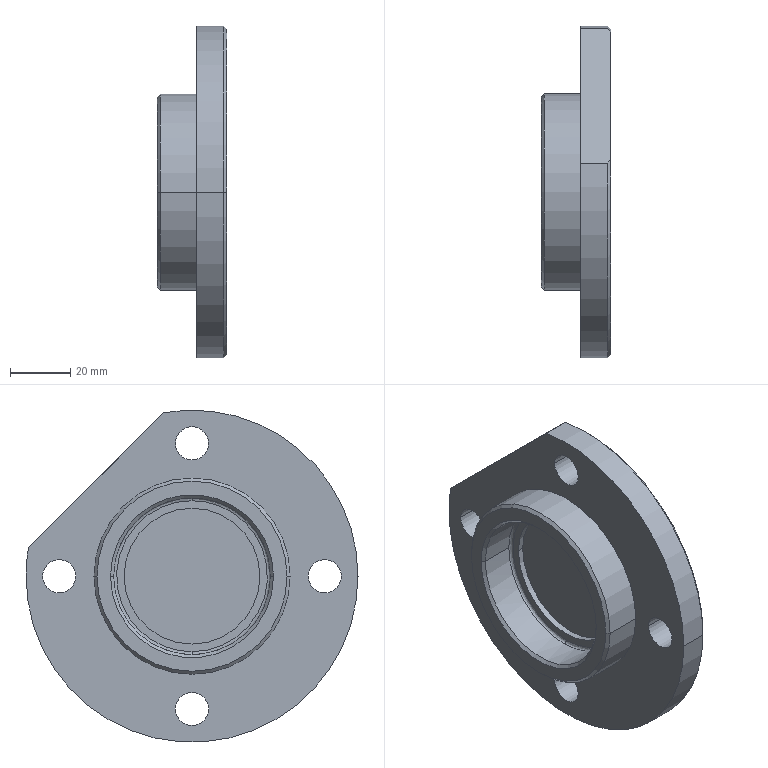Part | SolidWorks | features BaseBody 1 | 1 solid | 32 faces | box 23 x 110 x 110 mm | volume 98995 mm3 | cylinder 17 | cone 7 | plane 6 | spline 2 | commonest cylinder face diameters 11 x8 110 x3 45 x2 52 x2 65 x2